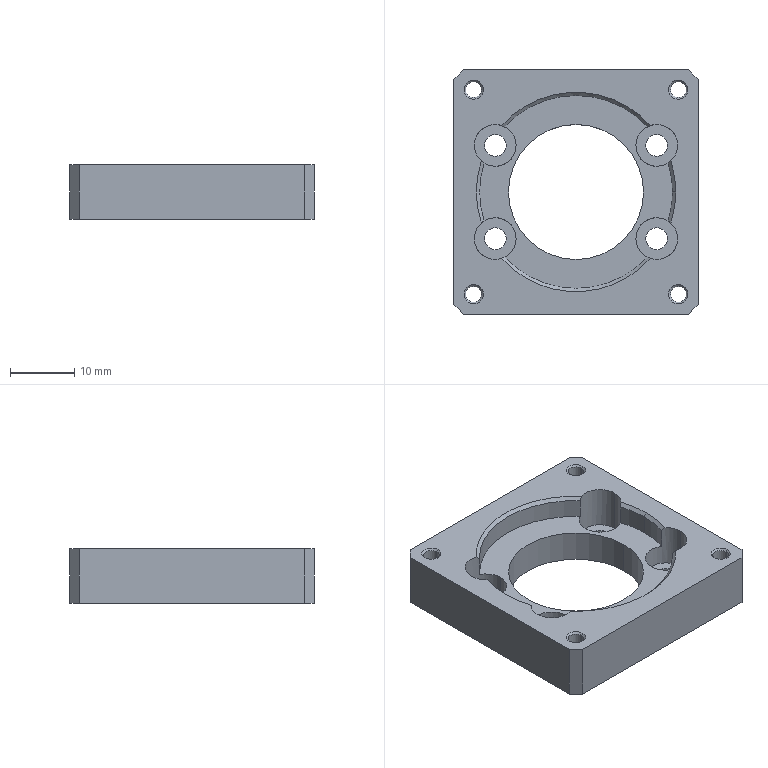Part | STEP file | QA-lx2001_A2038 | 1 solid | 67 faces | box 38 x 38 x 8.5 mm | volume 7170 mm3 | cylinder 31 | cone 21 | plane 15 | commonest cylinder face diameters 2.459 x8 3.4 x8 6.5 x8 30 x5 21 x2